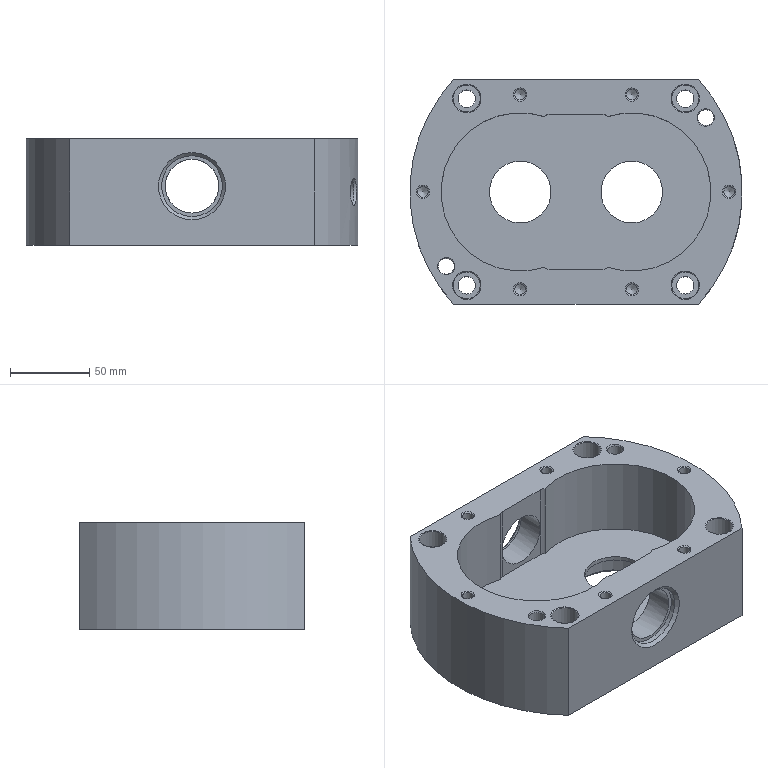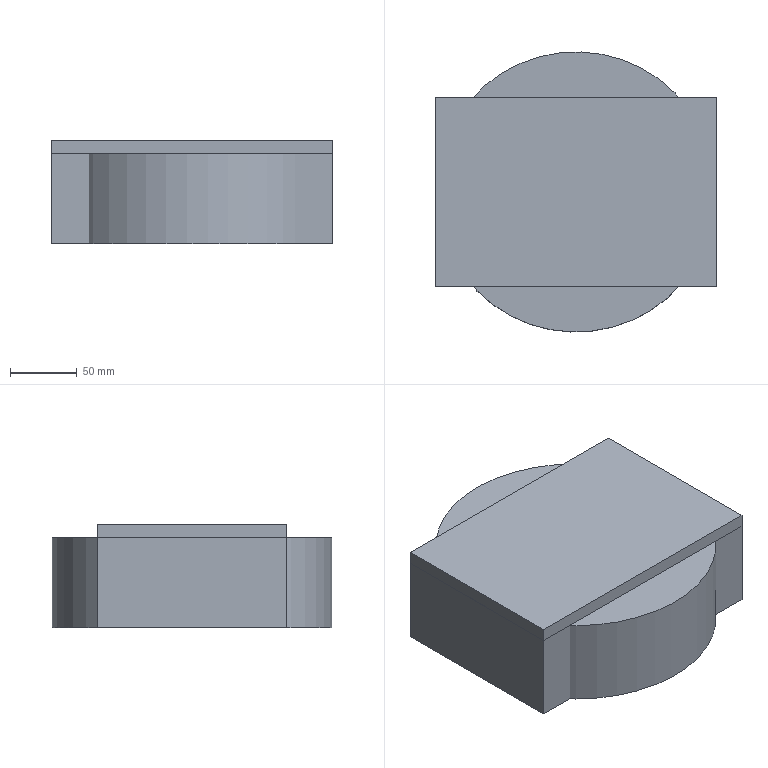CAM job | NX | 3+2 milling, drilling | part box 210 x 142 x 67.4 mm | stock box 210 x 210 x 77.4 mm
Tools:
number,name,description,diameter,corner_radius,flute_length,length,flutes
2,D50,Milling Tool-5 Parameters,50.0,0.0,50.0,75.0,2
10,D10,Milling Tool-5 Parameters,10.0,0.0,50.0,75.0,2
11,D10JING,Milling Tool-5 Parameters,10.0,0.0,50.0,75.0,2
7,D6A45,Milling Tool-5 Parameters,6.0,0.0,50.0,75.0,2
1,ZXZ,Milling Tool-5 Parameters,6.0,0.0,50.0,75.0,2
9,11.0ZT,Drilling Tool,11.0,0.0,35.0,50.0,2
19,9.8ZT,Drilling Tool,9.8,0.0,35.0,50.0,2
17,10.0JD,Milling Tool-5 Parameters,10.0,0.0,30.0,30.0,4
15,4.2ZT,Drilling Tool,4.2,0.0,35.0,50.0,2
14,M5,Milling Tool-5 Parameters,4.2,0.0,30.0,30.0,4
6,D6,Milling Tool-5 Parameters,6.0,0.0,50.0,75.0,2
8,D8,Milling Tool-5 Parameters,8.0,0.0,50.0,75.0,2
16,6.8ZT,Drilling Tool,6.8,0.0,35.0,50.0,2
18,M8,Milling Tool-5 Parameters,6.8,0.0,30.0,30.0,4
5,D25R0.5,Milling Tool-5 Parameters,25.0,0.5,50.0,75.0,2
12,D12,Milling Tool-5 Parameters,12.0,0.0,50.0,75.0,2
24,D100JD,Milling Tool-5 Parameters,100.0,0.0,30.0,30.0,4
Operations:
program,operation,operation_type,tool,method,geometry_group,spindle_rpm,surface_speed,feed_per_tooth,feed_cut,feed_plunge,cut_length_mm,path_length_mm,cut_time_min,machine_time_min
1,FLOOR_WALL,VolumeBased25DMillingOperation,D50,METHOD,A,1200.0,188.0,0.8333,2000.0,1000.0,59395.949,86797.827,29.989,32.729
1,FLOOR_WALL_COPY,VolumeBased25DMillingOperation,D50,METHOD,A,2500.0,392.0,0.2,1000.0,1000.0,753.535,875.535,0.7535,0.7657
1,HOLE_MILLING,CylinderMilling,D10,METHOD,A,3000.0,94.0,0.3667,2200.0,100.0,3134.936,3269.436,1.425,1.438
1,HOLE_MILLING_COPY,CylinderMilling,D10,METHOD,A,3000.0,94.0,0.3667,2200.0,100.0,3580.374,3736.374,1.627,1.643
1,HOLE_MILLING_COPY_1,CylinderMilling,D10JING,METHOD,A,5000.0,157.0,0.1,1000.0,100.0,121.857,259.857,0.1219,0.1357
1,HOLE_MILLING_COPY_1_COPY,CylinderMilling,D10JING,METHOD,A,5000.0,157.0,0.1,1000.0,100.0,113.097,285.097,0.1131,0.1303
1,PLANAR_MILL,PlanarMilling,D6A45,METHOD,A,7500.0,141.0,0.0833,1250.0,100.0,329.317,648.117,0.2635,0.2953
1,PLANAR_MILL_COPY,PlanarMilling,D6A45,METHOD,A,7500.0,141.0,0.0833,1250.0,100.0,360.844,487.844,0.2887,0.3014
2,DRILLING,Operation,ZXZ,METHOD,B,5000.0,94.0,0.025,250.0,0.0,64.0,774.131,0.256,0.327
2,DRILLING_COPY,Operation,11.0ZT,METHOD,B,2000.0,56.0,0.0375,150.0,0.0,294.819,1032.747,1.966,2.039
2,DRILLING_COPY_COPY,Operation,9.8ZT,METHOD,B,2000.0,56.0,0.0375,150.0,0.0,149.688,551.43,0.9979,1.038
2,DRILLING_COPY_COPY_COPY,Operation,10.0JD,METHOD,B,800.0,20.0,0.0125,40.0,0.0,141.8,535.653,3.545,3.584
2,DRILLING_COPY_COPY_1,Operation,4.2ZT,METHOD,B,2000.0,56.0,0.0375,150.0,0.0,138.095,651.822,0.9206,0.972
2,DRILLING_COPY_2_COPY_COPY_1_COPY,Operation,M5,METHOD,B,200.0,3.0,0.0009,0.7,0.0,128.0,631.633,182.857,182.907
2,HOLE_MILLING_COPY_COPY,CylinderMilling,D10,METHOD,B,3000.0,94.0,0.3667,2200.0,100.0,18887.046,19103.946,8.585,8.607
2,HOLE_MILLING_COPY_COPY_COPY,CylinderMilling,D10,METHOD,B,3000.0,94.0,0.3667,2200.0,100.0,7123.416,7376.716,3.238,3.263
2,FLOOR_WALL_1,VolumeBased25DMillingOperation,D10,METHOD,B,3000.0,94.0,0.3667,2200.0,1000.0,57496.397,58234.223,26.54,26.614
2,FLOOR_WALL_2,VolumeBased25DMillingOperation,D10JING,METHOD,B,5000.0,157.0,0.1,1000.0,100.0,5861.364,6501.216,5.861,5.925
2,ZLEVEL_PROFILE_COPY,ZLevelMilling,D6,METHOD,B,5000.0,94.0,0.16,1600.0,1000.0,9340.221,16534.998,6.745,7.465
2,ZLEVEL_PROFILE_COPY_COPY,ZLevelMilling,D8,METHOD,B,4500.0,84.0,0.1889,1700.0,1000.0,177865.691,179818.084,104.706,104.901
2,PLANAR_MILL_COPY_1,PlanarMilling,D6A45,METHOD,B,7500.0,141.0,0.0833,1250.0,100.0,850.858,1630.575,0.6807,0.7587
2,PLANAR_MILL_COPY_1_COPY,PlanarMilling,D6A45,METHOD,B,7500.0,141.0,0.0833,1250.0,100.0,929.804,1887.954,0.7438,0.8397
2,PLANAR_MILL_COPY_1_COPY_COPY,PlanarMilling,D6A45,METHOD,B,7500.0,141.0,0.0833,1250.0,100.0,249.225,527.011,0.1994,0.2272
2,CUTTER_COMP11,CylinderMilling,D10JING,METHOD,B,5000.0,157.0,0.1,1000.0,100.0,310.139,559.763,0.3101,0.3351
2,CUTTER_COMP_6,CylinderMilling,D6,METHOD,B,5000.0,157.0,0.1,1000.0,100.0,227.536,489.108,0.2275,0.2537
3,FLOOR_WALL_COPY_1,VolumeBased25DMillingOperation,D50,METHOD,C,1200.0,188.0,0.8333,2000.0,1000.0,45065.913,55289.613,22.62,23.642
3,FLOOR_WALL_COPY_COPY,VolumeBased25DMillingOperation,D50,METHOD,C,2500.0,392.0,0.2,1000.0,1000.0,1553.997,1607.997,1.554,1.559
3,DRILLING_COPY_1,Operation,ZXZ,METHOD,C,5000.0,94.0,0.025,250.0,0.0,24.0,525.205,0.096,0.1461
3,DRILLING_COPY_1_COPY,Operation,6.8ZT,METHOD,C,2000.0,42.0,0.05,200.0,0.0,150.258,777.72,0.7513,0.814
3,DRILLING_COPY_2_COPY_COPY,Operation,M8,METHOD,C,200.0,4.0,0.0016,1.25,0.0,138.0,753.205,110.4,110.462
3,FLOOR_WALL_1_1,VolumeBased25DMillingOperation,D25R0.5,METHOD,C,2000.0,157.0,0.55,2200.0,1000.0,138967.169,144095.874,68.712,69.225
3,ZLEVEL_PROFILE_COPY_COPY_1,ZLevelMilling,D8,METHOD,C,3740.0,94.0,0.2139,1600.0,1000.0,14375.363,23596.472,10.697,11.619
3,FLOOR_WALL_1_COPY_COPY,VolumeBased25DMillingOperation,D12,METHOD,C,4000.0,150.0,0.125,1000.0,500.0,2636.993,3014.126,2.647,2.684
3,ZLEVEL_PROFILE,ZLevelMilling,D12,METHOD,C,5000.0,157.0,0.125,1250.0,100.0,321.378,807.773,0.2571,0.3057
3,HOLE_MILLING_1,CylinderMilling,D10,METHOD,C,3500.0,109.0,0.3143,2200.0,100.0,11347.897,12059.897,5.158,5.229
3,PLANAR_MILL_COPY_1_COPY_1,PlanarMilling,D6A45,METHOD,C,7500.0,141.0,0.0833,1250.0,100.0,954.982,2273.213,0.764,0.8958
3,DRILLING_1,Operation,D100JD,METHOD,C,300.0,94.0,0.0417,50.0,0.0,106.4,346.364,2.128,2.152